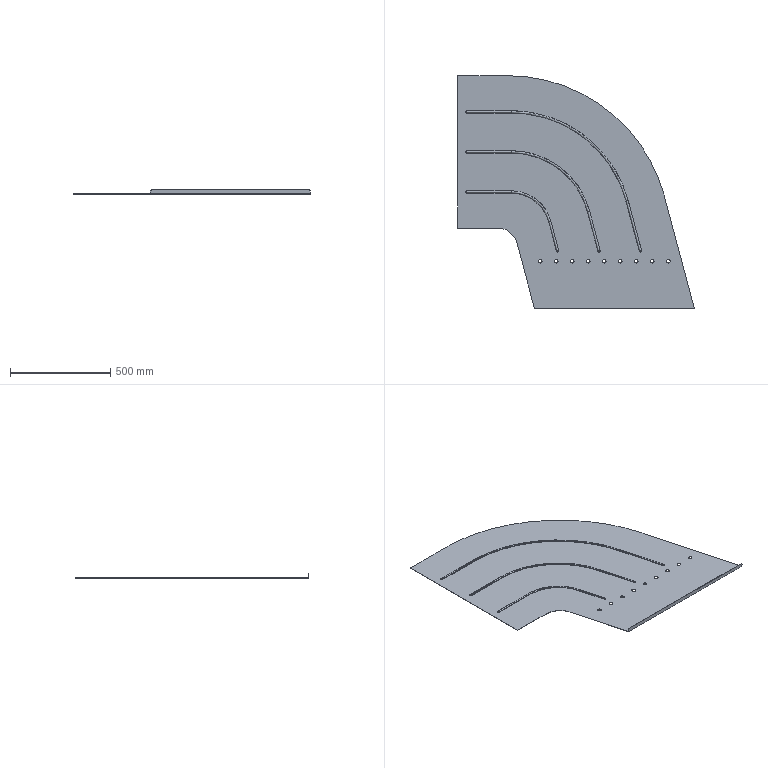Part | STEP file | 750078461 | 1 solid | 120 faces | box 1184 x 1163 x 20 mm | volume 1210389 mm3 | cylinder 60 | spline 48 | plane 12 | commonest cylinder face diameters 6 x18 8.4 x18 18 x18 10 x2 0.5 x1 2.9 x1